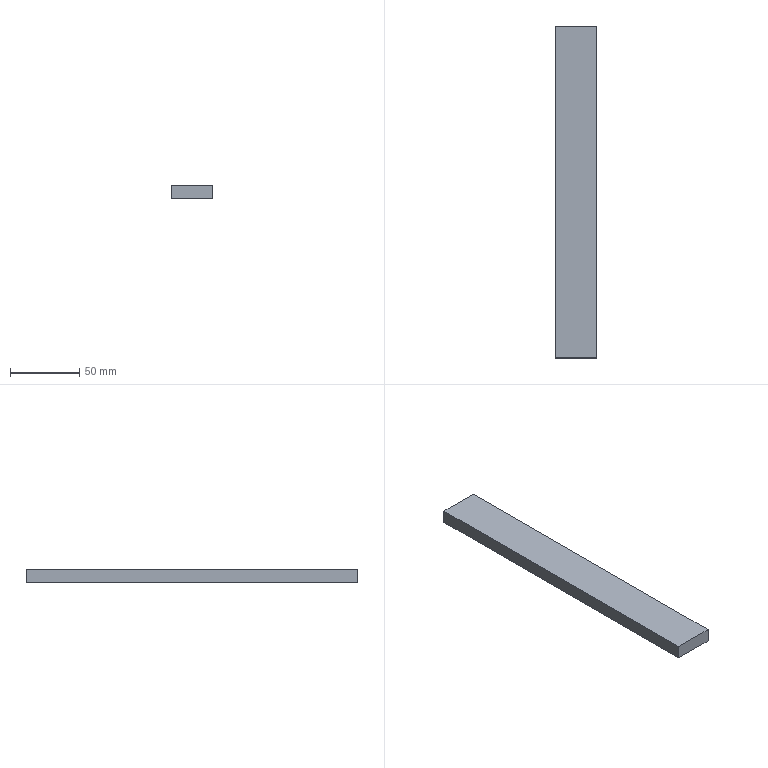Part | SolidWorks | features BaseBody 1 | 1 solid | 6 faces | box 30 x 240 x 10 mm | volume 72000 mm3 | plane 6
STEP:
#1=CARTESIAN_POINT('',(42.247,930.5,-356.997));
#2=VERTEX_POINT('',#1);
#3=CARTESIAN_POINT('',(72.247,930.5,-356.997));
#4=VERTEX_POINT('',#3);
#5=CARTESIAN_POINT('',(57.247,930.5,-356.997));
#6=DIRECTION('',(1.,0.,0.));
#7=VECTOR('',#6,1000.);
#8=LINE('',#5,#7);
#9=EDGE_CURVE('',#2,#4,#8,.T.);
#10=ORIENTED_EDGE('',*,*,#9,.F.);
#11=CARTESIAN_POINT('',(42.247,1170.5,-356.997));
#12=VERTEX_POINT('',#11);
#13=CARTESIAN_POINT('',(42.247,1050.5,-356.997));
#14=DIRECTION('',(0.,-1.,0.));
#15=VECTOR('',#14,1000.);
#16=LINE('',#13,#15);
#17=EDGE_CURVE('',#12,#2,#16,.T.);
#18=ORIENTED_EDGE('',*,*,#17,.F.);
#19=CARTESIAN_POINT('',(72.247,1170.5,-356.997));
#20=VERTEX_POINT('',#19);
#21=CARTESIAN_POINT('',(57.247,1170.5,-356.997));
#22=DIRECTION('',(-1.,0.,0.));
#23=VECTOR('',#22,1000.);
#24=LINE('',#21,#23);
#25=EDGE_CURVE('',#20,#12,#24,.T.);
#26=ORIENTED_EDGE('',*,*,#25,.F.);
#27=CARTESIAN_POINT('',(72.247,1050.5,-356.997));
#28=DIRECTION('',(0.,1.,0.));
#29=VECTOR('',#28,1000.);
#30=LINE('',#27,#29);
#31=EDGE_CURVE('',#4,#20,#30,.T.);
#32=ORIENTED_EDGE('',*,*,#31,.F.);
#33=EDGE_LOOP('',(#10,#18,#26,#32));
#34=FACE_OUTER_BOUND('',#33,.T.);
#35=CARTESIAN_POINT('',(57.247,1050.5,-356.997));
#36=DIRECTION('',(0.,0.,1.));
#37=DIRECTION('',(1.,0.,0.));
#38=AXIS2_PLACEMENT_3D('',#35,#36,#37);
#39=PLANE('',#38);
#40=ADVANCED_FACE('',(#34),#39,.F.);
#41=CARTESIAN_POINT('',(72.247,930.5,-346.997));
#42=VERTEX_POINT('',#41);
#43=CARTESIAN_POINT('',(72.247,1170.5,-346.997));
#44=VERTEX_POINT('',#43);
#45=CARTESIAN_POINT('',(72.247,930.5,-346.997));
#46=DIRECTION('',(0.,1.,0.));
#47=VECTOR('',#46,1000.);
#48=LINE('',#45,#47);
#49=EDGE_CURVE('',#42,#44,#48,.T.);
#50=ORIENTED_EDGE('',*,*,#49,.F.);
#51=CARTESIAN_POINT('',(72.247,930.5,-346.997));
#52=DIRECTION('',(0.,0.,1.));
#53=VECTOR('',#52,1000.);
#54=LINE('',#51,#53);
#55=EDGE_CURVE('',#4,#42,#54,.T.);
#56=ORIENTED_EDGE('',*,*,#55,.F.);
#57=ORIENTED_EDGE('',*,*,#31,.T.);
#58=CARTESIAN_POINT('',(72.247,1170.5,-346.997));
#59=DIRECTION('',(0.,0.,-1.));
#60=VECTOR('',#59,1000.);
#61=LINE('',#58,#60);
#62=EDGE_CURVE('',#44,#20,#61,.T.);
#63=ORIENTED_EDGE('',*,*,#62,.F.);
#64=EDGE_LOOP('',(#50,#56,#57,#63));
#65=FACE_OUTER_BOUND('',#64,.T.);
#66=CARTESIAN_POINT('',(72.247,930.5,-346.997));
#67=DIRECTION('',(-1.,0.,0.));
#68=DIRECTION('',(0.,0.,1.));
#69=AXIS2_PLACEMENT_3D('',#66,#67,#68);
#70=PLANE('',#69);
#71=ADVANCED_FACE('',(#65),#70,.F.);
#72=CARTESIAN_POINT('',(42.247,930.5,-346.997));
#73=VERTEX_POINT('',#72);
#74=CARTESIAN_POINT('',(42.247,930.5,-346.997));
#75=DIRECTION('',(1.,0.,0.));
#76=VECTOR('',#75,1000.);
#77=LINE('',#74,#76);
#78=EDGE_CURVE('',#73,#42,#77,.T.);
#79=ORIENTED_EDGE('',*,*,#78,.F.);
#80=CARTESIAN_POINT('',(42.247,930.5,-346.997));
#81=DIRECTION('',(0.,0.,1.));
#82=VECTOR('',#81,1000.);
#83=LINE('',#80,#82);
#84=EDGE_CURVE('',#2,#73,#83,.T.);
#85=ORIENTED_EDGE('',*,*,#84,.F.);
#86=ORIENTED_EDGE('',*,*,#9,.T.);
#87=ORIENTED_EDGE('',*,*,#55,.T.);
#88=EDGE_LOOP('',(#79,#85,#86,#87));
#89=FACE_OUTER_BOUND('',#88,.T.);
#90=CARTESIAN_POINT('',(42.247,930.5,-346.997));
#91=DIRECTION('',(0.,1.,0.));
#92=DIRECTION('',(0.,0.,1.));
#93=AXIS2_PLACEMENT_3D('',#90,#91,#92);
#94=PLANE('',#93);
#95=ADVANCED_FACE('',(#89),#94,.F.);
#96=CARTESIAN_POINT('',(42.247,1170.5,-346.997));
#97=VERTEX_POINT('',#96);
#98=CARTESIAN_POINT('',(42.247,930.5,-346.997));
#99=DIRECTION('',(0.,-1.,0.));
#100=VECTOR('',#99,1000.);
#101=LINE('',#98,#100);
#102=EDGE_CURVE('',#97,#73,#101,.T.);
#103=ORIENTED_EDGE('',*,*,#102,.F.);
#104=CARTESIAN_POINT('',(42.247,1170.5,-346.997));
#105=DIRECTION('',(0.,0.,1.));
#106=VECTOR('',#105,1000.);
#107=LINE('',#104,#106);
#108=EDGE_CURVE('',#12,#97,#107,.T.);
#109=ORIENTED_EDGE('',*,*,#108,.F.);
#110=ORIENTED_EDGE('',*,*,#17,.T.);
#111=ORIENTED_EDGE('',*,*,#84,.T.);
#112=EDGE_LOOP('',(#103,#109,#110,#111));
#113=FACE_OUTER_BOUND('',#112,.T.);
#114=CARTESIAN_POINT('',(42.247,930.5,-346.997));
#115=DIRECTION('',(1.,0.,0.));
#116=DIRECTION('',(0.,0.,-1.));
#117=AXIS2_PLACEMENT_3D('',#114,#115,#116);
#118=PLANE('',#117);
#119=ADVANCED_FACE('',(#113),#118,.F.);
#120=CARTESIAN_POINT('',(42.247,1170.5,-346.997));
#121=DIRECTION('',(-1.,0.,0.));
#122=VECTOR('',#121,1000.);
#123=LINE('',#120,#122);
#124=EDGE_CURVE('',#44,#97,#123,.T.);
#125=ORIENTED_EDGE('',*,*,#124,.F.);
#126=ORIENTED_EDGE('',*,*,#62,.T.);
#127=ORIENTED_EDGE('',*,*,#25,.T.);
#128=ORIENTED_EDGE('',*,*,#108,.T.);
#129=EDGE_LOOP('',(#125,#126,#127,#128));
#130=FACE_OUTER_BOUND('',#129,.T.);
#131=CARTESIAN_POINT('',(42.247,1170.5,-346.997));
#132=DIRECTION('',(0.,-1.,0.));
#133=DIRECTION('',(0.,0.,-1.));
#134=AXIS2_PLACEMENT_3D('',#131,#132,#133);
#135=PLANE('',#134);
#136=ADVANCED_FACE('',(#130),#135,.F.);
#137=ORIENTED_EDGE('',*,*,#49,.T.);
#138=ORIENTED_EDGE('',*,*,#124,.T.);
#139=ORIENTED_EDGE('',*,*,#102,.T.);
#140=ORIENTED_EDGE('',*,*,#78,.T.);
#141=EDGE_LOOP('',(#137,#138,#139,#140));
#142=FACE_OUTER_BOUND('',#141,.T.);
#143=CARTESIAN_POINT('',(57.247,1050.5,-346.997));
#144=DIRECTION('',(0.,0.,1.));
#145=DIRECTION('',(1.,0.,0.));
#146=AXIS2_PLACEMENT_3D('',#143,#144,#145);
#147=PLANE('',#146);
#148=ADVANCED_FACE('',(#142),#147,.T.);
#149=CLOSED_SHELL('',(#40,#71,#95,#119,#136,#148));
#150=MANIFOLD_SOLID_BREP('',#149);
#151=CARTESIAN_POINT('',(0.,0.,0.));
#152=DIRECTION('',(0.,0.,1.));
#153=DIRECTION('',(1.,0.,0.));
#154=AXIS2_PLACEMENT_3D('',#151,#152,#153);
#155=(LENGTH_UNIT()NAMED_UNIT(*)SI_UNIT(.MILLI.,.METRE.));
#156=UNCERTAINTY_MEASURE_WITH_UNIT(LENGTH_MEASURE(0.00001),#155,'','');
#157=(NAMED_UNIT(*)PLANE_ANGLE_UNIT()SI_UNIT($,.RADIAN.));
#158=(NAMED_UNIT(*)SI_UNIT($,.STERADIAN.)SOLID_ANGLE_UNIT());
#159=(GEOMETRIC_REPRESENTATION_CONTEXT(3)GLOBAL_UNCERTAINTY_ASSIGNED_CONTEXT((#156))GLOBAL_UNIT_ASSIGNED_CONTEXT((#155,#157,#158))REPRESENTATION_CONTEXT('',''));
#160=ADVANCED_BREP_SHAPE_REPRESENTATION('',(#150,#154),#159);